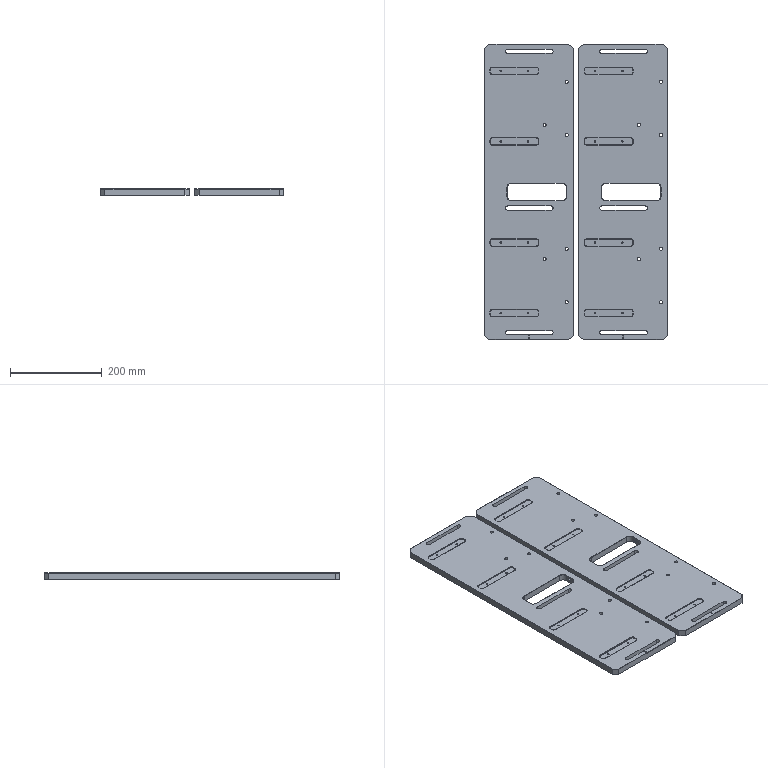NC program | NX | posted by the shop | part box 401 x 645 x 14 mm
Lines 1 to 1341 of 5636:
%
O0001
(Machine time: 77.76 MIN)
(===Total Tool:4===)
(T9=D10     D=10.  R=0.   D-  H09 Z=0.5   )
(T6=D6      D=6.   R=0.   D-  H06 Z=0.2   )
(T7=D6-J    D=6.   R=0.   D7  H07 Z=0.2   )
(T2=D6 chamfer mill   D=6.   R=0.   D-  H02 Z=9.85  )
G80 G90 G17 G49 G40
G91 G28 Z0
M01
N1 T09 M06
(D10  D=10. R=0. H=09 ce=0.10 di=0.10)
G00 G90 G54 X-108.113 Y112.409 M03 S6000
G43 H09 Z34.
M08
Z14.5
M03 S6000
G01 Y134.5 Z13.729 F2800.
X-107.813
M03 S6000
Y182.5 F3500.
X-107.816 Y182.549
X-107.851 Y182.584
X-107.9 Y182.587
X-113.1
X-113.149 Y182.584
X-113.184 Y182.549
X-113.187 Y182.5
Y86.5
X-113.184 Y86.451
X-113.149 Y86.416
X-113.1 Y86.413
X-107.9
X-107.851 Y86.416
X-107.816 Y86.451
X-107.813 Y86.5
Y134.5
Z14.729
G00 Z15.
X-108.3 Y112.409
Z14.229
M03 S6000
G01 Y134.5 Z13.457 F2800.
X-108.
M03 S6000
Y182.4 F3500.
X-113.
Y86.6
X-108.
Y134.5
Z14.457
G00 Z14.729
X-108.3 Y112.409
Z13.957
M03 S6000
G01 Y134.5 Z13.186 F2800.
X-108.
M03 S6000
Y182.4 F3500.
X-113.
Y86.6
X-108.
Y134.5
Z14.186
G00 Z14.457
X-108.3 Y112.409
Z13.686
M03 S6000
G01 Y134.5 Z12.914 F2800.
X-108.
M03 S6000
Y182.4 F3500.
X-113.
Y86.6
X-108.
Y134.5
Z13.914
G00 Z14.186
X-108.3 Y112.409
Z13.414
M03 S6000
G01 Y134.5 Z12.643 F2800.
X-108.
M03 S6000
Y182.4 F3500.
X-113.
Y86.6
X-108.
Y134.5
Z13.643
G00 Z13.914
X-108.3 Y112.409
Z13.143
M03 S6000
G01 Y134.5 Z12.371 F2800.
X-108.
M03 S6000
Y182.4 F3500.
X-113.
Y86.6
X-108.
Y134.5
Z13.371
G00 Z13.643
X-108.3 Y112.409
Z12.871
M03 S6000
G01 Y134.5 Z12.1 F2800.
X-108.
M03 S6000
Y182.4 F3500.
X-113.
Y86.6
X-108.
Y134.5
Z13.1
G00 Z34.
X-266.887 Y156.591
Z14.5
M03 S6000
G01 Y134.5 Z13.729 F2800.
X-267.187
M03 S6000
Y86.5 F3500.
X-267.184 Y86.451
X-267.149 Y86.416
X-267.1 Y86.413
X-261.9
X-261.851 Y86.416
X-261.816 Y86.451
X-261.813 Y86.5
Y182.5
X-261.816 Y182.549
X-261.851 Y182.584
X-261.9 Y182.587
X-267.1
X-267.149 Y182.584
X-267.184 Y182.549
X-267.187 Y182.5
Y134.5
Z14.729
G00 Z15.
X-266.7 Y156.591
Z14.229
M03 S6000
G01 Y134.5 Z13.457 F2800.
X-267.
M03 S6000
Y86.6 F3500.
X-262.
Y182.4
X-267.
Y134.5
Z14.457
G00 Z14.729
X-266.7 Y156.591
Z13.957
M03 S6000
G01 Y134.5 Z13.186 F2800.
X-267.
M03 S6000
Y86.6 F3500.
X-262.
Y182.4
X-267.
Y134.5
Z14.186
G00 Z14.457
X-266.7 Y156.591
Z13.686
M03 S6000
G01 Y134.5 Z12.914 F2800.
X-267.
M03 S6000
Y86.6 F3500.
X-262.
Y182.4
X-267.
Y134.5
Z13.914
G00 Z14.186
X-266.7 Y156.591
Z13.414
M03 S6000
G01 Y134.5 Z12.643 F2800.
X-267.
M03 S6000
Y86.6 F3500.
X-262.
Y182.4
X-267.
Y134.5
Z13.643
G00 Z13.914
X-266.7 Y156.591
Z13.143
M03 S6000
G01 Y134.5 Z12.371 F2800.
X-267.
M03 S6000
Y86.6 F3500.
X-262.
Y182.4
X-267.
Y134.5
Z13.371
G00 Z13.643
X-266.7 Y156.591
Z12.871
M03 S6000
G01 Y134.5 Z12.1 F2800.
X-267.
M03 S6000
Y86.6 F3500.
X-262.
Y182.4
X-267.
Y134.5
Z13.1
G00 Z34.
X-266.887 Y-49.409
Z14.5
M03 S6000
G01 Y-71.5 Z13.729 F2800.
X-267.187
M03 S6000
Y-119.5 F3500.
X-267.184 Y-119.549
X-267.149 Y-119.584
X-267.1 Y-119.587
X-261.9
X-261.851 Y-119.584
X-261.816 Y-119.549
X-261.813 Y-119.5
Y-23.5
X-261.816 Y-23.451
X-261.851 Y-23.416
X-261.9 Y-23.413
X-267.1
X-267.149 Y-23.416
X-267.184 Y-23.451
X-267.187 Y-23.5
Y-71.5
Z14.729
G00 Z15.
X-266.7 Y-49.409
Z14.229
M03 S6000
G01 Y-71.5 Z13.457 F2800.
X-267.
M03 S6000
Y-119.4 F3500.
X-262.
Y-23.6
X-267.
Y-71.5
Z14.457
G00 Z14.729
X-266.7 Y-49.409
Z13.957
M03 S6000
G01 Y-71.5 Z13.186 F2800.
X-267.
M03 S6000
Y-119.4 F3500.
X-262.
Y-23.6
X-267.
Y-71.5
Z14.186
G00 Z14.457
X-266.7 Y-49.409
Z13.686
M03 S6000
G01 Y-71.5 Z12.914 F2800.
X-267.
M03 S6000
Y-119.4 F3500.
X-262.
Y-23.6
X-267.
Y-71.5
Z13.914
G00 Z14.186
X-266.7 Y-49.409
Z13.414
M03 S6000
G01 Y-71.5 Z12.643 F2800.
X-267.
M03 S6000
Y-119.4 F3500.
X-262.
Y-23.6
X-267.
Y-71.5
Z13.643
G00 Z13.914
X-266.7 Y-49.409
Z13.143
M03 S6000
G01 Y-71.5 Z12.371 F2800.
X-267.
M03 S6000
Y-119.4 F3500.
X-262.
Y-23.6
X-267.
Y-71.5
Z13.371
G00 Z13.643
X-266.7 Y-49.409
Z12.871
M03 S6000
G01 Y-71.5 Z12.1 F2800.
X-267.
M03 S6000
Y-119.4 F3500.
X-262.
Y-23.6
X-267.
Y-71.5
Z13.1
G00 Z34.
X-112.887 Y-49.409
Z14.5
M03 S6000
G01 Y-71.5 Z13.729 F2800.
X-113.187
M03 S6000
Y-119.5 F3500.
X-113.184 Y-119.549
X-113.149 Y-119.584
X-113.1 Y-119.587
X-107.9
X-107.851 Y-119.584
X-107.816 Y-119.549
X-107.813 Y-119.5
Y-23.5
X-107.816 Y-23.451
X-107.851 Y-23.416
X-107.9 Y-23.413
X-113.1
X-113.149 Y-23.416
X-113.184 Y-23.451
X-113.187 Y-23.5
Y-71.5
Z14.729
G00 Z15.
X-112.7 Y-49.409
Z14.229
M03 S6000
G01 Y-71.5 Z13.457 F2800.
X-113.
M03 S6000
Y-119.4 F3500.
X-108.
Y-23.6
X-113.
Y-71.5
Z14.457
G00 Z14.729
X-112.7 Y-49.409
Z13.957
M03 S6000
G01 Y-71.5 Z13.186 F2800.
X-113.
M03 S6000
Y-119.4 F3500.
X-108.
Y-23.6
X-113.
Y-71.5
Z14.186
G00 Z14.457
X-112.7 Y-49.409
Z13.686
M03 S6000
G01 Y-71.5 Z12.914 F2800.
X-113.
M03 S6000
Y-119.4 F3500.
X-108.
Y-23.6
X-113.
Y-71.5
Z13.914
G00 Z14.186
X-112.7 Y-49.409
Z13.414
M03 S6000
G01 Y-71.5 Z12.643 F2800.
X-113.
M03 S6000
Y-119.4 F3500.
X-108.
Y-23.6
X-113.
Y-71.5
Z13.643
G00 Z13.914
X-112.7 Y-49.409
Z13.143
M03 S6000
G01 Y-71.5 Z12.371 F2800.
X-113.
M03 S6000
Y-119.4 F3500.
X-108.
Y-23.6
X-113.
Y-71.5
Z13.371
G00 Z13.643
X-112.7 Y-49.409
Z12.871
M03 S6000
G01 Y-71.5 Z12.1 F2800.
X-113.
M03 S6000
Y-119.4 F3500.
X-108.
Y-23.6
X-113.
Y-71.5
Z13.1
G00 Z34.
X108.113 Y-49.409
Z14.5
M03 S6000
G01 Y-71.5 Z13.729 F2800.
X107.813
M03 S6000
Y-119.5 F3500.
X107.816 Y-119.549
X107.851 Y-119.584
X107.9 Y-119.587
X113.1
X113.149 Y-119.584
X113.184 Y-119.549
X113.187 Y-119.5
Y-23.5
X113.184 Y-23.451
X113.149 Y-23.416
X113.1 Y-23.413
X107.9
X107.851 Y-23.416
X107.816 Y-23.451
X107.813 Y-23.5
Y-71.5
Z14.729
G00 Z15.
X108.3 Y-49.409
Z14.229
M03 S6000
G01 Y-71.5 Z13.457 F2800.
X108.
M03 S6000
Y-119.4 F3500.
X113.
Y-23.6
X108.
Y-71.5
Z14.457
G00 Z14.729
X108.3 Y-49.409
Z13.957
M03 S6000
G01 Y-71.5 Z13.186 F2800.
X108.
M03 S6000
Y-119.4 F3500.
X113.
Y-23.6
X108.
Y-71.5
Z14.186
G00 Z14.457
X108.3 Y-49.409
Z13.686
M03 S6000
G01 Y-71.5 Z12.914 F2800.
X108.
M03 S6000
Y-119.4 F3500.
X113.
Y-23.6
X108.
Y-71.5
Z13.914
G00 Z14.186
X108.3 Y-49.409
Z13.414
M03 S6000
G01 Y-71.5 Z12.643 F2800.
X108.
M03 S6000
Y-119.4 F3500.
X113.
Y-23.6
X108.
Y-71.5
Z13.643
G00 Z13.914
X108.3 Y-49.409
Z13.143
M03 S6000
G01 Y-71.5 Z12.371 F2800.
X108.
M03 S6000
Y-119.4 F3500.
X113.
Y-23.6
X108.
Y-71.5
Z13.371
G00 Z13.643
X108.3 Y-49.409
Z12.871
M03 S6000
G01 Y-71.5 Z12.1 F2800.
X108.
M03 S6000
Y-119.4 F3500.
X113.
Y-23.6
X108.
Y-71.5
Z13.1
G00 Z34.
X266.887 Y-93.591
Z14.5
M03 S6000
G01 Y-71.5 Z13.729 F2800.
X267.187
M03 S6000
Y-23.5 F3500.
X267.184 Y-23.451
X267.149 Y-23.416
X267.1 Y-23.413
X261.9
X261.851 Y-23.416
X261.816 Y-23.451
X261.813 Y-23.5
Y-119.5
X261.816 Y-119.549
X261.851 Y-119.584
X261.9 Y-119.587
X267.1
X267.149 Y-119.584
X267.184 Y-119.549
X267.187 Y-119.5
Y-71.5
Z14.729
G00 Z15.
X266.7 Y-93.591
Z14.229
M03 S6000
G01 Y-71.5 Z13.457 F2800.
X267.
M03 S6000
Y-23.6 F3500.
X262.
Y-119.4
X267.
Y-71.5
Z14.457
G00 Z14.729
X266.7 Y-93.591
Z13.957
M03 S6000
G01 Y-71.5 Z13.186 F2800.
X267.
M03 S6000
Y-23.6 F3500.
X262.
Y-119.4
X267.
Y-71.5
Z14.186
G00 Z14.457
X266.7 Y-93.591
Z13.686
M03 S6000
G01 Y-71.5 Z12.914 F2800.
X267.
M03 S6000
Y-23.6 F3500.
X262.
Y-119.4
X267.
Y-71.5
Z13.914
G00 Z14.186
X266.7 Y-93.591
Z13.414
M03 S6000
G01 Y-71.5 Z12.643 F2800.
X267.
M03 S6000
Y-23.6 F3500.
X262.
Y-119.4
X267.
Y-71.5
Z13.643
G00 Z13.914
X266.7 Y-93.591
Z13.143
M03 S6000
G01 Y-71.5 Z12.371 F2800.
X267.
M03 S6000
Y-23.6 F3500.
X262.
Y-119.4
X267.
Y-71.5
Z13.371
G00 Z13.643
X266.7 Y-93.591
Z12.871
M03 S6000
G01 Y-71.5 Z12.1 F2800.
X267.
M03 S6000
Y-23.6 F3500.
X262.
Y-119.4
X267.
Y-71.5
Z13.1
G00 Z34.
X266.887 Y112.409
Z14.5
M03 S6000
G01 Y134.5 Z13.729 F2800.
X267.187
M03 S6000
Y182.5 F3500.
X267.184 Y182.549
X267.149 Y182.584
X267.1 Y182.587
X261.9
X261.851 Y182.584
X261.816 Y182.549
X261.813 Y182.5
Y86.5
X261.816 Y86.451
X261.851 Y86.416
X261.9 Y86.413
X267.1
X267.149 Y86.416
X267.184 Y86.451
X267.187 Y86.5
Y134.5
Z14.729
G00 Z15.
X266.7 Y112.409
Z14.229
M03 S6000
G01 Y134.5 Z13.457 F2800.
X267.
M03 S6000
Y182.4 F3500.
X262.
Y86.6
X267.
Y134.5
Z14.457
G00 Z14.729
X266.7 Y112.409
Z13.957
M03 S6000
G01 Y134.5 Z13.186 F2800.
X267.
M03 S6000
Y182.4 F3500.
X262.
Y86.6
X267.
Y134.5
Z14.186
G00 Z14.457
X266.7 Y112.409
Z13.686
M03 S6000
G01 Y134.5 Z12.914 F2800.
X267.
M03 S6000
Y182.4 F3500.
X262.
Y86.6
X267.
Y134.5
Z13.914
G00 Z14.186
X266.7 Y112.409
Z13.414
M03 S6000
G01 Y134.5 Z12.643 F2800.
X267.
M03 S6000
Y182.4 F3500.
X262.
Y86.6
X267.
Y134.5
Z13.643
G00 Z13.914
X266.7 Y112.409
Z13.143
M03 S6000
G01 Y134.5 Z12.371 F2800.
X267.
M03 S6000
Y182.4 F3500.
X262.
Y86.6
X267.
Y134.5
Z13.371
G00 Z13.643
X266.7 Y112.409
Z12.871
M03 S6000
G01 Y134.5 Z12.1 F2800.
X267.
M03 S6000
Y182.4 F3500.
X262.
Y86.6
X267.
Y134.5
Z13.1
G00 Z34.
X112.887 Y112.409
Z14.5
M03 S6000
G01 Y134.5 Z13.729 F2800.
X113.187
M03 S6000
Y182.5 F3500.
X113.184 Y182.549
X113.149 Y182.584
X113.1 Y182.587
X107.9
X107.851 Y182.584
X107.816 Y182.549
X107.813 Y182.5
Y86.5
X107.816 Y86.451
X107.851 Y86.416
X107.9 Y86.413
X113.1
X113.149 Y86.416
X113.184 Y86.451
X113.187 Y86.5
Y134.5
Z14.729
G00 Z15.
X112.7 Y112.409
Z14.229
M03 S6000
G01 Y134.5 Z13.457 F2800.
X113.
M03 S6000
Y182.4 F3500.
X108.
Y86.6
X113.
Y134.5
Z14.457
G00 Z14.729
X112.7 Y112.409
Z13.957
M03 S6000
G01 Y134.5 Z13.186 F2800.
X113.
M03 S6000
Y182.4 F3500.
X108.
Y86.6
X113.
Y134.5
Z14.186
G00 Z14.457
X112.7 Y112.409
Z13.686
M03 S6000
G01 Y134.5 Z12.914 F2800.
X113.
M03 S6000
Y182.4 F3500.
X108.
Y86.6
X113.
Y134.5
Z13.914
G00 Z14.186
X112.7 Y112.409
Z13.414
M03 S6000
G01 Y134.5 Z12.643 F2800.
X113.
M03 S6000
Y182.4 F3500.
X108.
Y86.6
X113.
Y134.5
Z13.643
G00 Z13.914
X112.7 Y112.409
Z13.143
M03 S6000
G01 Y134.5 Z12.371 F2800.
X113.
M03 S6000
Y182.4 F3500.
X108.
Y86.6
X113.
Y134.5
Z13.371
G00 Z13.643
X112.7 Y112.409
Z12.871
M03 S6000
G01 Y134.5 Z12.1 F2800.
X113.
M03 S6000
Y182.4 F3500.
X108.
Y86.6
X113.
Y134.5
Z13.1
G00 Z34.
G00 G90 X-13.9 Y85.5 M03 S6000
Z34.
Z14.5
G01 Y30.5 Z14.407 F4000.
G03 X-9. Y25.6 Z14.394 I4.9 J0.0
G01 X9. Z14.364
G03 X13.9 Y30.5 Z14.351 I0.0 J4.9
G01 Y140.5 Z14.166
G03 X9. Y145.4 Z14.153 I-4.9 J0.0
G01 X-9. Z14.123
G03 X-13.9 Y140.5 Z14.11 I0.0 J-4.9
G01 Y30.5 Z13.925
G03 X-9. Y25.6 Z13.912 I4.9 J0.0
G01 X9. Z13.881
G03 X13.9 Y30.5 Z13.868 I0.0 J4.9
G01 Y140.5 Z13.683
G03 X9. Y145.4 Z13.67 I-4.9 J0.0
G01 X-9. Z13.64
G03 X-13.9 Y140.5 Z13.627 I0.0 J-4.9
G01 Y30.5 Z13.442
G03 X-9. Y25.6 Z13.429 I4.9 J0.0
G01 X9. Z13.399
G03 X13.9 Y30.5 Z13.386 I0.0 J4.9
G01 Y140.5 Z13.201
G03 X9. Y145.4 Z13.188 I-4.9 J0.0
G01 X-9. Z13.157
G03 X-13.9 Y140.5 Z13.144 I0.0 J-4.9
G01 Y30.5 Z12.959
G03 X-9. Y25.6 Z12.946 I4.9 J0.0
G01 X9. Z12.916
G03 X13.9 Y30.5 Z12.903 I0.0 J4.9
G01 Y140.5 Z12.718
G03 X9. Y145.4 Z12.705 I-4.9 J0.0
G01 X-9. Z12.675
G03 X-13.9 Y140.5 Z12.662 I0.0 J-4.9
G01 Y30.5 Z12.476
G03 X-9. Y25.6 Z12.463 I4.9 J0.0
G01 X9. Z12.433
G03 X13.9 Y30.5 Z12.42 I0.0 J4.9
G01 Y140.5 Z12.235
G03 X9. Y145.4 Z12.222 I-4.9 J0.0
G01 X-9. Z12.192
G03 X-13.9 Y140.5 Z12.179 I0.0 J-4.9
G01 Y30.5 Z11.994
G03 X-9. Y25.6 Z11.981 I4.9 J0.0
G01 X9. Z11.95
G03 X13.9 Y30.5 Z11.937 I0.0 J4.9
G01 Y140.5 Z11.752
G03 X9. Y145.4 Z11.739 I-4.9 J0.0
G01 X-9. Z11.709
G03 X-13.9 Y140.5 Z11.696 I0.0 J-4.9
G01 Y30.5 Z11.511
G03 X-9. Y25.6 Z11.498 I4.9 J0.0
G01 X9. Z11.468
G03 X13.9 Y30.5 Z11.455 I0.0 J4.9
G01 Y140.5 Z11.269
G03 X9. Y145.4 Z11.257 I-4.9 J0.0
G01 X-9. Z11.226
G03 X-13.9 Y140.5 Z11.213 I0.0 J-4.9
G01 Y30.5 Z11.028
G03 X-9. Y25.6 Z11.015 I4.9 J0.0
G01 X9. Z10.985
G03 X13.9 Y30.5 Z10.972 I0.0 J4.9
G01 Y140.5 Z10.787
G03 X9. Y145.4 Z10.774 I-4.9 J0.0
G01 X-9. Z10.743
G03 X-13.9 Y140.5 Z10.731 I0.0 J-4.9
G01 Y30.5 Z10.545
G03 X-9. Y25.6 Z10.532 I4.9 J0.0
G01 X9. Z10.502
G03 X13.9 Y30.5 Z10.489 I0.0 J4.9
G01 Y140.5 Z10.304
G03 X9. Y145.4 Z10.291 I-4.9 J0.0
G01 X-9. Z10.261
G03 X-13.9 Y140.5 Z10.248 I0.0 J-4.9
G01 Y30.5 Z10.063
G03 X-9. Y25.6 Z10.05 I4.9 J0.0
G01 X9. Z10.019
G03 X13.9 Y30.5 Z10.006 I0.0 J4.9
G01 Y140.5 Z9.821
G03 X9. Y145.4 Z9.808 I-4.9 J0.0
G01 X-9. Z9.778
G03 X-13.9 Y140.5 Z9.765 I0.0 J-4.9
G01 Y30.5 Z9.58
G03 X-9. Y25.6 Z9.567 I4.9 J0.0
G01 X9. Z9.537
G03 X13.9 Y30.5 Z9.524 I0.0 J4.9
G01 Y140.5 Z9.338
G03 X9. Y145.4 Z9.325 I-4.9 J0.0
G01 X-9. Z9.295
G03 X-13.9 Y140.5 Z9.282 I0.0 J-4.9
G01 Y30.5 Z9.097
G03 X-9. Y25.6 Z9.084 I4.9 J0.0
G01 X9. Z9.054
G03 X13.9 Y30.5 Z9.041 I0.0 J4.9
G01 Y140.5 Z8.856
G03 X9. Y145.4 Z8.843 I-4.9 J0.0
G01 X-9. Z8.812
G03 X-13.9 Y140.5 Z8.799 I0.0 J-4.9
G01 Y30.5 Z8.614
G03 X-9. Y25.6 Z8.601 I4.9 J0.0
G01 X9. Z8.571
G03 X13.9 Y30.5 Z8.558 I0.0 J4.9
G01 Y140.5 Z8.373
G03 X9. Y145.4 Z8.36 I-4.9 J0.0
G01 X-9. Z8.33
G03 X-13.9 Y140.5 Z8.317 I0.0 J-4.9
G01 Y30.5 Z8.132
G03 X-9. Y25.6 Z8.119 I4.9 J0.0
G01 X9. Z8.088
G03 X13.9 Y30.5 Z8.075 I0.0 J4.9
G01 Y140.5 Z7.89
G03 X9. Y145.4 Z7.877 I-4.9 J0.0
G01 X-9. Z7.847
G03 X-13.9 Y140.5 Z7.834 I0.0 J-4.9
G01 Y30.5 Z7.649
G03 X-9. Y25.6 Z7.636 I4.9 J0.0
G01 X9. Z7.606
G03 X13.9 Y30.5 Z7.593 I0.0 J4.9
G01 Y140.5 Z7.407
G03 X9. Y145.4 Z7.394 I-4.9 J0.0
G01 X-9. Z7.364
G03 X-13.9 Y140.5 Z7.351 I0.0 J-4.9
G01 Y30.5 Z7.166
G03 X-9. Y25.6 Z7.153 I4.9 J0.0
G01 X9. Z7.123
G03 X13.9 Y30.5 Z7.11 I0.0 J4.9
G01 Y140.5 Z6.925
G03 X9. Y145.4 Z6.912 I-4.9 J0.0
G01 X-9. Z6.881
G03 X-13.9 Y140.5 Z6.868 I0.0 J-4.9
G01 Y30.5 Z6.683
G03 X-9. Y25.6 Z6.67 I4.9 J0.0
G01 X9. Z6.64
G03 X13.9 Y30.5 Z6.627 I0.0 J4.9
G01 Y140.5 Z6.442
G03 X9. Y145.4 Z6.429 I-4.9 J0.0
G01 X-9. Z6.399
G03 X-13.9 Y140.5 Z6.386 I0.0 J-4.9
G01 Y30.5 Z6.201
G03 X-9. Y25.6 Z6.188 I4.9 J0.0
G01 X9. Z6.157
G03 X13.9 Y30.5 Z6.144 I0.0 J4.9
G01 Y140.5 Z5.959
G03 X9. Y145.4 Z5.946 I-4.9 J0.0
G01 X-9. Z5.916
G03 X-13.9 Y140.5 Z5.903 I0.0 J-4.9
G01 Y30.5 Z5.718
G03 X-9. Y25.6 Z5.705 I4.9 J0.0
G01 X9. Z5.675
G03 X13.9 Y30.5 Z5.662 I0.0 J4.9
G01 Y140.5 Z5.476
G03 X9. Y145.4 Z5.463 I-4.9 J0.0
G01 X-9. Z5.433
G03 X-13.9 Y140.5 Z5.42 I0.0 J-4.9
G01 Y30.5 Z5.235
G03 X-9. Y25.6 Z5.222 I4.9 J0.0
G01 X9. Z5.192
G03 X13.9 Y30.5 Z5.179 I0.0 J4.9
G01 Y140.5 Z4.994
G03 X9. Y145.4 Z4.981 I-4.9 J0.0
G01 X-9. Z4.95
G03 X-13.9 Y140.5 Z4.937 I0.0 J-4.9
G01 Y30.5 Z4.752
G03 X-9. Y25.6 Z4.739 I4.9 J0.0
G01 X9. Z4.709
G03 X13.9 Y30.5 Z4.696 I0.0 J4.9
G01 Y140.5 Z4.511
G03 X9. Y145.4 Z4.498 I-4.9 J0.0
G01 X-9. Z4.468
G03 X-13.9 Y140.5 Z4.455 I0.0 J-4.9
G01 Y30.5 Z4.269
G03 X-9. Y25.6 Z4.257 I4.9 J0.0
G01 X9. Z4.226
G03 X13.9 Y30.5 Z4.213 I0.0 J4.9
G01 Y140.5 Z4.028
G03 X9. Y145.4 Z4.015 I-4.9 J0.0
G01 X-9. Z3.985
G03 X-13.9 Y140.5 Z3.972 I0.0 J-4.9
G01 Y30.5 Z3.787
G03 X-9. Y25.6 Z3.774 I4.9 J0.0
G01 X9. Z3.743
G03 X13.9 Y30.5 Z3.731 I0.0 J4.9
G01 Y140.5 Z3.545
G03 X9. Y145.4 Z3.532 I-4.9 J0.0
G01 X-9. Z3.502
G03 X-13.9 Y140.5 Z3.489 I0.0 J-4.9
G01 Y30.5 Z3.304
G03 X-9. Y25.6 Z3.291 I4.9 J0.0
G01 X9. Z3.261
G03 X13.9 Y30.5 Z3.248 I0.0 J4.9
G01 Y140.5 Z3.063
G03 X9. Y145.4 Z3.05 I-4.9 J0.0
G01 X-9. Z3.019
G03 X-13.9 Y140.5 Z3.006 I0.0 J-4.9
G01 Y30.5 Z2.821
G03 X-9. Y25.6 Z2.808 I4.9 J0.0
G01 X9. Z2.778
G03 X13.9 Y30.5 Z2.765 I0.0 J4.9
G01 Y140.5 Z2.58
G03 X9. Y145.4 Z2.567 I-4.9 J0.0
G01 X-9. Z2.537
G03 X-13.9 Y140.5 Z2.524 I0.0 J-4.9
G01 Y30.5 Z2.338
G03 X-9. Y25.6 Z2.325 I4.9 J0.0
G01 X9. Z2.295
G03 X13.9 Y30.5 Z2.282 I0.0 J4.9
G01 Y140.5 Z2.097
G03 X9. Y145.4 Z2.084 I-4.9 J0.0
G01 X-9. Z2.054
G03 X-13.9 Y140.5 Z2.041 I0.0 J-4.9
G01 Y30.5 Z1.856
G03 X-9. Y25.6 Z1.843 I4.9 J0.0
G01 X9. Z1.812
G03 X13.9 Y30.5 Z1.799 I0.0 J4.9
G01 Y140.5 Z1.614
G03 X9. Y145.4 Z1.601 I-4.9 J0.0
G01 X-9. Z1.571
G03 X-13.9 Y140.5 Z1.558 I0.0 J-4.9
G01 Y30.5 Z1.373
G03 X-9. Y25.6 Z1.36 I4.9 J0.0
G01 X9. Z1.33
G03 X13.9 Y30.5 Z1.317 I0.0 J4.9
G01 Y140.5 Z1.132
G03 X9. Y145.4 Z1.119 I-4.9 J0.0
G01 X-9. Z1.088
G03 X-13.9 Y140.5 Z1.075 I0.0 J-4.9
G01 Y30.5 Z.89
G03 X-9. Y25.6 Z.877 I4.9 J0.0
G01 X9. Z.847
G03 X13.9 Y30.5 Z.834 I0.0 J4.9
G01 Y140.5 Z.649
G03 X9. Y145.4 Z.636 I-4.9 J0.0
G01 X-9. Z.606
G03 X-13.9 Y140.5 Z.593 I0.0 J-4.9
G01 Y85.5 Z.5
Y30.5
G03 X-9. Y25.6 I4.9 J0.0
G01 X9.
G03 X13.9 Y30.5 I0.0 J4.9
G01 Y140.5
G03 X9. Y145.4 I-4.9 J0.0
G01 X-9.
G03 X-13.9 Y140.5 I0.0 J-4.9
G01 Y85.5
Y85.
Z1.5
G00 Z34.
Y-120.5
Z14.5
G01 Y-175.5 Z14.407
G03 X-9. Y-180.4 Z14.394 I4.9 J0.0
G01 X9. Z14.364
G03 X13.9 Y-175.5 Z14.351 I0.0 J4.9
G01 Y-65.5 Z14.166
G03 X9. Y-60.6 Z14.153 I-4.9 J0.0
G01 X-9. Z14.123
G03 X-13.9 Y-65.5 Z14.11 I0.0 J-4.9
G01 Y-175.5 Z13.925
G03 X-9. Y-180.4 Z13.912 I4.9 J0.0
G01 X9. Z13.881
G03 X13.9 Y-175.5 Z13.868 I0.0 J4.9
G01 Y-65.5 Z13.683
G03 X9. Y-60.6 Z13.67 I-4.9 J0.0
G01 X-9. Z13.64
G03 X-13.9 Y-65.5 Z13.627 I0.0 J-4.9
G01 Y-175.5 Z13.442
G03 X-9. Y-180.4 Z13.429 I4.9 J0.0
G01 X9. Z13.399
G03 X13.9 Y-175.5 Z13.386 I0.0 J4.9
G01 Y-65.5 Z13.201
G03 X9. Y-60.6 Z13.188 I-4.9 J0.0
G01 X-9. Z13.157
G03 X-13.9 Y-65.5 Z13.144 I0.0 J-4.9
G01 Y-175.5 Z12.959
G03 X-9. Y-180.4 Z12.946 I4.9 J0.0
G01 X9. Z12.916
G03 X13.9 Y-175.5 Z12.903 I0.0 J4.9
G01 Y-65.5 Z12.718
G03 X9. Y-60.6 Z12.705 I-4.9 J0.0
G01 X-9. Z12.675
G03 X-13.9 Y-65.5 Z12.662 I0.0 J-4.9
G01 Y-175.5 Z12.476
G03 X-9. Y-180.4 Z12.463 I4.9 J0.0
G01 X9. Z12.433
G03 X13.9 Y-175.5 Z12.42 I0.0 J4.9
G01 Y-65.5 Z12.235
G03 X9. Y-60.6 Z12.222 I-4.9 J0.0
G01 X-9. Z12.192
G03 X-13.9 Y-65.5 Z12.179 I0.0 J-4.9
G01 Y-175.5 Z11.994
G03 X-9. Y-180.4 Z11.981 I4.9 J0.0
G01 X9. Z11.95
G03 X13.9 Y-175.5 Z11.937 I0.0 J4.9
G01 Y-65.5 Z11.752
G03 X9. Y-60.6 Z11.739 I-4.9 J0.0
G01 X-9. Z11.709
G03 X-13.9 Y-65.5 Z11.696 I0.0 J-4.9
G01 Y-175.5 Z11.511
G03 X-9. Y-180.4 Z11.498 I4.9 J0.0
G01 X9. Z11.468
G03 X13.9 Y-175.5 Z11.455 I0.0 J4.9
G01 Y-65.5 Z11.269
G03 X9. Y-60.6 Z11.257 I-4.9 J0.0
G01 X-9. Z11.226
G03 X-13.9 Y-65.5 Z11.213 I0.0 J-4.9
G01 Y-175.5 Z11.028
G03 X-9. Y-180.4 Z11.015 I4.9 J0.0
G01 X9. Z10.985
G03 X13.9 Y-175.5 Z10.972 I0.0 J4.9
G01 Y-65.5 Z10.787
G03 X9. Y-60.6 Z10.774 I-4.9 J0.0
G01 X-9. Z10.743
G03 X-13.9 Y-65.5 Z10.731 I0.0 J-4.9
G01 Y-175.5 Z10.545
G03 X-9. Y-180.4 Z10.532 I4.9 J0.0
G01 X9. Z10.502
G03 X13.9 Y-175.5 Z10.489 I0.0 J4.9
G01 Y-65.5 Z10.304
G03 X9. Y-60.6 Z10.291 I-4.9 J0.0
G01 X-9. Z10.261
G03 X-13.9 Y-65.5 Z10.248 I0.0 J-4.9
G01 Y-175.5 Z10.063
G03 X-9. Y-180.4 Z10.05 I4.9 J0.0
G01 X9. Z10.019
G03 X13.9 Y-175.5 Z10.006 I0.0 J4.9
G01 Y-65.5 Z9.821
G03 X9. Y-60.6 Z9.808 I-4.9 J0.0
G01 X-9. Z9.778
G03 X-13.9 Y-65.5 Z9.765 I0.0 J-4.9
G01 Y-175.5 Z9.58
G03 X-9. Y-180.4 Z9.567 I4.9 J0.0
G01 X9. Z9.537
G03 X13.9 Y-175.5 Z9.524 I0.0 J4.9
G01 Y-65.5 Z9.338
G03 X9. Y-60.6 Z9.325 I-4.9 J0.0
G01 X-9. Z9.295
G03 X-13.9 Y-65.5 Z9.282 I0.0 J-4.9
G01 Y-175.5 Z9.097
G03 X-9. Y-180.4 Z9.084 I4.9 J0.0
G01 X9. Z9.054
G03 X13.9 Y-175.5 Z9.041 I0.0 J4.9
G01 Y-65.5 Z8.856
G03 X9. Y-60.6 Z8.843 I-4.9 J0.0
G01 X-9. Z8.812
G03 X-13.9 Y-65.5 Z8.799 I0.0 J-4.9
G01 Y-175.5 Z8.614
G03 X-9. Y-180.4 Z8.601 I4.9 J0.0
G01 X9. Z8.571
G03 X13.9 Y-175.5 Z8.558 I0.0 J4.9
G01 Y-65.5 Z8.373
G03 X9. Y-60.6 Z8.36 I-4.9 J0.0
G01 X-9. Z8.33
G03 X-13.9 Y-65.5 Z8.317 I0.0 J-4.9
G01 Y-175.5 Z8.132
G03 X-9. Y-180.4 Z8.119 I4.9 J0.0
G01 X9. Z8.088
G03 X13.9 Y-175.5 Z8.075 I0.0 J4.9
G01 Y-65.5 Z7.89
G03 X9. Y-60.6 Z7.877 I-4.9 J0.0
G01 X-9. Z7.847
G03 X-13.9 Y-65.5 Z7.834 I0.0 J-4.9
G01 Y-175.5 Z7.649
G03 X-9. Y-180.4 Z7.636 I4.9 J0.0
G01 X9. Z7.606
G03 X13.9 Y-175.5 Z7.593 I0.0 J4.9
G01 Y-65.5 Z7.407
G03 X9. Y-60.6 Z7.394 I-4.9 J0.0
G01 X-9. Z7.364
G03 X-13.9 Y-65.5 Z7.351 I0.0 J-4.9
G01 Y-175.5 Z7.166
G03 X-9. Y-180.4 Z7.153 I4.9 J0.0
G01 X9. Z7.123
G03 X13.9 Y-175.5 Z7.11 I0.0 J4.9
G01 Y-65.5 Z6.925
G03 X9. Y-60.6 Z6.912 I-4.9 J0.0
G01 X-9. Z6.881
G03 X-13.9 Y-65.5 Z6.868 I0.0 J-4.9
G01 Y-175.5 Z6.683
G03 X-9. Y-180.4 Z6.67 I4.9 J0.0
G01 X9. Z6.64
G03 X13.9 Y-175.5 Z6.627 I0.0 J4.9
G01 Y-65.5 Z6.442
G03 X9. Y-60.6 Z6.429 I-4.9 J0.0
G01 X-9. Z6.399
G03 X-13.9 Y-65.5 Z6.386 I0.0 J-4.9
G01 Y-175.5 Z6.201
G03 X-9. Y-180.4 Z6.188 I4.9 J0.0
G01 X9. Z6.157
G03 X13.9 Y-175.5 Z6.144 I0.0 J4.9
G01 Y-65.5 Z5.959
G03 X9. Y-60.6 Z5.946 I-4.9 J0.0
G01 X-9. Z5.916
G03 X-13.9 Y-65.5 Z5.903 I0.0 J-4.9
G01 Y-175.5 Z5.718
G03 X-9. Y-180.4 Z5.705 I4.9 J0.0
G01 X9. Z5.675
G03 X13.9 Y-175.5 Z5.662 I0.0 J4.9
G01 Y-65.5 Z5.476
G03 X9. Y-60.6 Z5.463 I-4.9 J0.0
G01 X-9. Z5.433
G03 X-13.9 Y-65.5 Z5.42 I0.0 J-4.9
G01 Y-175.5 Z5.235
G03 X-9. Y-180.4 Z5.222 I4.9 J0.0
G01 X9. Z5.192
G03 X13.9 Y-175.5 Z5.179 I0.0 J4.9
G01 Y-65.5 Z4.994
G03 X9. Y-60.6 Z4.981 I-4.9 J0.0
G01 X-9. Z4.95
G03 X-13.9 Y-65.5 Z4.937 I0.0 J-4.9
G01 Y-175.5 Z4.752
G03 X-9. Y-180.4 Z4.739 I4.9 J0.0
G01 X9. Z4.709
G03 X13.9 Y-175.5 Z4.696 I0.0 J4.9
G01 Y-65.5 Z4.511
G03 X9. Y-60.6 Z4.498 I-4.9 J0.0
G01 X-9. Z4.468
G03 X-13.9 Y-65.5 Z4.455 I0.0 J-4.9
G01 Y-175.5 Z4.269
G03 X-9. Y-180.4 Z4.257 I4.9 J0.0
G01 X9. Z4.226
G03 X13.9 Y-175.5 Z4.213 I0.0 J4.9
G01 Y-65.5 Z4.028
G03 X9. Y-60.6 Z4.015 I-4.9 J0.0
G01 X-9. Z3.985
G03 X-13.9 Y-65.5 Z3.972 I0.0 J-4.9
G01 Y-175.5 Z3.787
G03 X-9. Y-180.4 Z3.774 I4.9 J0.0
G01 X9. Z3.743
G03 X13.9 Y-175.5 Z3.731 I0.0 J4.9
G01 Y-65.5 Z3.545
G03 X9. Y-60.6 Z3.532 I-4.9 J0.0
G01 X-9. Z3.502
G03 X-13.9 Y-65.5 Z3.489 I0.0 J-4.9
G01 Y-175.5 Z3.304
G03 X-9. Y-180.4 Z3.291 I4.9 J0.0
G01 X9. Z3.261
G03 X13.9 Y-175.5 Z3.248 I0.0 J4.9
G01 Y-65.5 Z3.063
G03 X9. Y-60.6 Z3.05 I-4.9 J0.0
G01 X-9. Z3.019
G03 X-13.9 Y-65.5 Z3.006 I0.0 J-4.9
G01 Y-175.5 Z2.821
G03 X-9. Y-180.4 Z2.808 I4.9 J0.0
G01 X9. Z2.778
G03 X13.9 Y-175.5 Z2.765 I0.0 J4.9
G01 Y-65.5 Z2.58
G03 X9. Y-60.6 Z2.567 I-4.9 J0.0
G01 X-9. Z2.537
G03 X-13.9 Y-65.5 Z2.524 I0.0 J-4.9
G01 Y-175.5 Z2.338
G03 X-9. Y-180.4 Z2.325 I4.9 J0.0
G01 X9. Z2.295
G03 X13.9 Y-175.5 Z2.282 I0.0 J4.9
G01 Y-65.5 Z2.097
G03 X9. Y-60.6 Z2.084 I-4.9 J0.0
G01 X-9. Z2.054
G03 X-13.9 Y-65.5 Z2.041 I0.0 J-4.9
G01 Y-175.5 Z1.856
G03 X-9. Y-180.4 Z1.843 I4.9 J0.0
G01 X9. Z1.812
G03 X13.9 Y-175.5 Z1.799 I0.0 J4.9
G01 Y-65.5 Z1.614
G03 X9. Y-60.6 Z1.601 I-4.9 J0.0
G01 X-9. Z1.571
G03 X-13.9 Y-65.5 Z1.558 I0.0 J-4.9
G01 Y-175.5 Z1.373
G03 X-9. Y-180.4 Z1.36 I4.9 J0.0
G01 X9. Z1.33
G03 X13.9 Y-175.5 Z1.317 I0.0 J4.9
G01 Y-65.5 Z1.132
G03 X9. Y-60.6 Z1.119 I-4.9 J0.0
G01 X-9. Z1.088
G03 X-13.9 Y-65.5 Z1.075 I0.0 J-4.9
G01 Y-175.5 Z.89
G03 X-9. Y-180.4 Z.877 I4.9 J0.0
G01 X9. Z.847
G03 X13.9 Y-175.5 Z.834 I0.0 J4.9
G01 Y-65.5 Z.649
G03 X9. Y-60.6 Z.636 I-4.9 J0.0
G01 X-9. Z.606
G03 X-13.9 Y-65.5 Z.593 I0.0 J-4.9
G01 Y-120.5 Z.5
Y-175.5
G03 X-9. Y-180.4 I4.9 J0.0
G01 X9.
G03 X13.9 Y-175.5 I0.0 J4.9
G01 Y-65.5
G03 X9. Y-60.6 I-4.9 J0.0
G01 X-9.
G03 X-13.9 Y-65.5 I0.0 J-4.9
G01 Y-120.5
Y-121.
Z1.5
G00 Z34.
G91 G28 Z0.0
M05
M09
G91 G28 Z0.0
M01